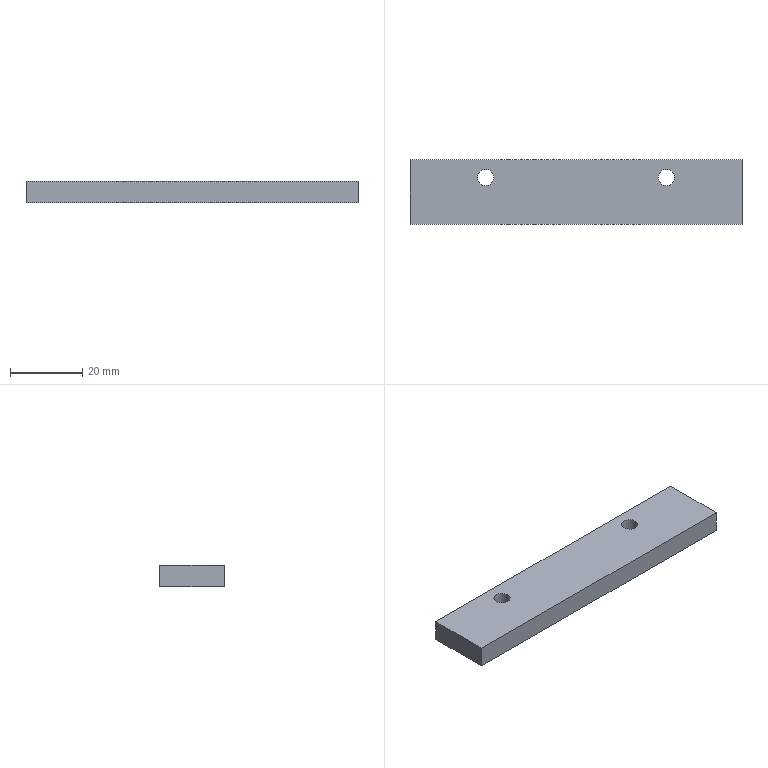Part | STEP file | 2061 Bag feed artificial stone plate A | 1 solid | 10 faces | box 92 x 18 x 6 mm | volume 9745 mm3 | plane 6 | cylinder 4 | commonest cylinder face diameters 4.5 x4
STEP:
#1=CARTESIAN_POINT('',(0.,0.,0.));
#2=DIRECTION('',(0.,0.,1.));
#3=DIRECTION('',(1.,0.,0.));
#4=AXIS2_PLACEMENT_3D('',#1,#2,#3);
#5=CARTESIAN_POINT('',(-22.75,4.,0.));
#6=VERTEX_POINT('',#5);
#7=CARTESIAN_POINT('',(-22.75,4.,6.));
#8=VERTEX_POINT('',#7);
#9=CARTESIAN_POINT('',(-22.75,4.,6.));
#10=DIRECTION('',(0.,0.,1.));
#11=VECTOR('',#10,1.);
#12=LINE('',#9,#11);
#13=CARTESIAN_POINT('',(-25.,4.,6.));
#14=DIRECTION('',(0.,0.,1.));
#15=DIRECTION('',(1.,0.,0.));
#16=AXIS2_PLACEMENT_3D('',#13,#14,#15);
#17=CYLINDRICAL_SURFACE('',#16,2.25);
#18=CARTESIAN_POINT('',(6.283,0.));
#19=DIRECTION('',(0.,1.));
#20=VECTOR('',#19,1.);
#21=LINE('',#18,#20);
#22=(GEOMETRIC_REPRESENTATION_CONTEXT(2)PARAMETRIC_REPRESENTATION_CONTEXT()REPRESENTATION_CONTEXT('',''));
#23=DEFINITIONAL_REPRESENTATION('',(#21),#22);
#24=PCURVE('',#17,#23);
#25=CARTESIAN_POINT('',(-25.,4.,6.));
#26=DIRECTION('',(0.,0.,1.));
#27=DIRECTION('',(1.,0.,0.));
#28=AXIS2_PLACEMENT_3D('',#25,#26,#27);
#29=CYLINDRICAL_SURFACE('',#28,2.25);
#30=CARTESIAN_POINT('',(0.,0.));
#31=DIRECTION('',(0.,1.));
#32=VECTOR('',#31,1.);
#33=LINE('',#30,#32);
#34=(GEOMETRIC_REPRESENTATION_CONTEXT(2)PARAMETRIC_REPRESENTATION_CONTEXT()REPRESENTATION_CONTEXT('',''));
#35=DEFINITIONAL_REPRESENTATION('',(#33),#34);
#36=PCURVE('',#29,#35);
#37=SURFACE_CURVE('',#12,(#24,#36),.PCURVE_S1.);
#38=EDGE_CURVE('',#6,#8,#37,.T.);
#39=ORIENTED_EDGE('',*,*,#38,.T.);
#40=CARTESIAN_POINT('',(-27.25,4.,6.));
#41=VERTEX_POINT('',#40);
#42=CARTESIAN_POINT('',(-25.,4.,6.));
#43=DIRECTION('',(0.,0.,1.));
#44=DIRECTION('',(1.,0.,0.));
#45=AXIS2_PLACEMENT_3D('',#42,#43,#44);
#46=CIRCLE('',#45,2.25);
#47=CARTESIAN_POINT('',(0.,0.));
#48=DIRECTION('',(1.,0.));
#49=VECTOR('',#48,1.);
#50=LINE('',#47,#49);
#51=(GEOMETRIC_REPRESENTATION_CONTEXT(2)PARAMETRIC_REPRESENTATION_CONTEXT()REPRESENTATION_CONTEXT('',''));
#52=DEFINITIONAL_REPRESENTATION('',(#50),#51);
#53=PCURVE('',#17,#52);
#54=CARTESIAN_POINT('',(0.,0.,6.));
#55=DIRECTION('',(0.,0.,-1.));
#56=DIRECTION('',(-1.,0.,0.));
#57=AXIS2_PLACEMENT_3D('',#54,#55,#56);
#58=PLANE('',#57);
#59=CARTESIAN_POINT('',(22.75,4.));
#60=CARTESIAN_POINT('',(22.75,7.897));
#61=CARTESIAN_POINT('',(26.125,5.949));
#62=CARTESIAN_POINT('',(29.5,4.));
#63=CARTESIAN_POINT('',(26.125,2.051));
#64=CARTESIAN_POINT('',(22.75,0.1029));
#65=CARTESIAN_POINT('',(22.75,4.));
#66=(BOUNDED_CURVE()B_SPLINE_CURVE(2,(#59,#60,#61,#62,#63,#64,#65),.UNSPECIFIED.,.T.,.F.)B_SPLINE_CURVE_WITH_KNOTS((1,2,2,2,2,1),(-2.094,0.,2.094,4.189,6.283,8.378),.UNSPECIFIED.)CURVE()GEOMETRIC_REPRESENTATION_ITEM()RATIONAL_B_SPLINE_CURVE((1.,0.5,1.,0.5,1.,0.5,1.))REPRESENTATION_ITEM(''));
#67=(GEOMETRIC_REPRESENTATION_CONTEXT(2)PARAMETRIC_REPRESENTATION_CONTEXT()REPRESENTATION_CONTEXT('',''));
#68=DEFINITIONAL_REPRESENTATION('',(#66),#67);
#69=PCURVE('',#58,#68);
#70=SURFACE_CURVE('',#46,(#53,#69),.PCURVE_S1.);
#71=EDGE_CURVE('',#41,#8,#70,.T.);
#72=ORIENTED_EDGE('',*,*,#71,.F.);
#73=CARTESIAN_POINT('',(-27.25,4.,0.));
#74=VERTEX_POINT('',#73);
#75=CARTESIAN_POINT('',(-27.25,4.,6.));
#76=DIRECTION('',(0.,0.,1.));
#77=VECTOR('',#76,1.);
#78=LINE('',#75,#77);
#79=CARTESIAN_POINT('',(3.142,0.));
#80=DIRECTION('',(0.,1.));
#81=VECTOR('',#80,1.);
#82=LINE('',#79,#81);
#83=(GEOMETRIC_REPRESENTATION_CONTEXT(2)PARAMETRIC_REPRESENTATION_CONTEXT()REPRESENTATION_CONTEXT('',''));
#84=DEFINITIONAL_REPRESENTATION('',(#82),#83);
#85=PCURVE('',#17,#84);
#86=CARTESIAN_POINT('',(3.142,0.));
#87=DIRECTION('',(0.,1.));
#88=VECTOR('',#87,1.);
#89=LINE('',#86,#88);
#90=(GEOMETRIC_REPRESENTATION_CONTEXT(2)PARAMETRIC_REPRESENTATION_CONTEXT()REPRESENTATION_CONTEXT('',''));
#91=DEFINITIONAL_REPRESENTATION('',(#89),#90);
#92=PCURVE('',#29,#91);
#93=SURFACE_CURVE('',#78,(#85,#92),.PCURVE_S1.);
#94=EDGE_CURVE('',#74,#41,#93,.T.);
#95=ORIENTED_EDGE('',*,*,#94,.F.);
#96=CARTESIAN_POINT('',(-25.,4.,0.));
#97=DIRECTION('',(0.,0.,-1.));
#98=DIRECTION('',(-1.,0.,0.));
#99=AXIS2_PLACEMENT_3D('',#96,#97,#98);
#100=CIRCLE('',#99,2.25);
#101=CARTESIAN_POINT('',(9.425,-6.));
#102=DIRECTION('',(-1.,0.));
#103=VECTOR('',#102,1.);
#104=LINE('',#101,#103);
#105=(GEOMETRIC_REPRESENTATION_CONTEXT(2)PARAMETRIC_REPRESENTATION_CONTEXT()REPRESENTATION_CONTEXT('',''));
#106=DEFINITIONAL_REPRESENTATION('',(#104),#105);
#107=PCURVE('',#17,#106);
#108=CARTESIAN_POINT('',(0.,0.,0.));
#109=DIRECTION('',(0.,0.,-1.));
#110=DIRECTION('',(-1.,0.,0.));
#111=AXIS2_PLACEMENT_3D('',#108,#109,#110);
#112=PLANE('',#111);
#113=CARTESIAN_POINT('',(25.,4.));
#114=DIRECTION('',(1.,0.));
#115=AXIS2_PLACEMENT_2D('',#113,#114);
#116=CIRCLE('',#115,2.25);
#117=(GEOMETRIC_REPRESENTATION_CONTEXT(2)PARAMETRIC_REPRESENTATION_CONTEXT()REPRESENTATION_CONTEXT('',''));
#118=DEFINITIONAL_REPRESENTATION('',(#116),#117);
#119=PCURVE('',#112,#118);
#120=SURFACE_CURVE('',#100,(#107,#119),.PCURVE_S1.);
#121=EDGE_CURVE('',#6,#74,#120,.T.);
#122=ORIENTED_EDGE('',*,*,#121,.F.);
#123=EDGE_LOOP('',(#39,#72,#95,#122));
#124=FACE_BOUND('',#123,.F.);
#125=ADVANCED_FACE('',(#124),#17,.F.);
#126=CARTESIAN_POINT('',(27.25,4.,0.));
#127=VERTEX_POINT('',#126);
#128=CARTESIAN_POINT('',(27.25,4.,6.));
#129=VERTEX_POINT('',#128);
#130=CARTESIAN_POINT('',(27.25,4.,6.));
#131=DIRECTION('',(0.,0.,1.));
#132=VECTOR('',#131,1.);
#133=LINE('',#130,#132);
#134=CARTESIAN_POINT('',(25.,4.,6.));
#135=DIRECTION('',(0.,0.,1.));
#136=DIRECTION('',(1.,0.,0.));
#137=AXIS2_PLACEMENT_3D('',#134,#135,#136);
#138=CYLINDRICAL_SURFACE('',#137,2.25);
#139=CARTESIAN_POINT('',(6.283,0.));
#140=DIRECTION('',(0.,1.));
#141=VECTOR('',#140,1.);
#142=LINE('',#139,#141);
#143=(GEOMETRIC_REPRESENTATION_CONTEXT(2)PARAMETRIC_REPRESENTATION_CONTEXT()REPRESENTATION_CONTEXT('',''));
#144=DEFINITIONAL_REPRESENTATION('',(#142),#143);
#145=PCURVE('',#138,#144);
#146=CARTESIAN_POINT('',(25.,4.,6.));
#147=DIRECTION('',(0.,0.,1.));
#148=DIRECTION('',(1.,0.,0.));
#149=AXIS2_PLACEMENT_3D('',#146,#147,#148);
#150=CYLINDRICAL_SURFACE('',#149,2.25);
#151=CARTESIAN_POINT('',(0.,0.));
#152=DIRECTION('',(0.,1.));
#153=VECTOR('',#152,1.);
#154=LINE('',#151,#153);
#155=(GEOMETRIC_REPRESENTATION_CONTEXT(2)PARAMETRIC_REPRESENTATION_CONTEXT()REPRESENTATION_CONTEXT('',''));
#156=DEFINITIONAL_REPRESENTATION('',(#154),#155);
#157=PCURVE('',#150,#156);
#158=SURFACE_CURVE('',#133,(#145,#157),.PCURVE_S1.);
#159=EDGE_CURVE('',#127,#129,#158,.T.);
#160=ORIENTED_EDGE('',*,*,#159,.T.);
#161=CARTESIAN_POINT('',(22.75,4.,6.));
#162=VERTEX_POINT('',#161);
#163=CARTESIAN_POINT('',(25.,4.,6.));
#164=DIRECTION('',(0.,0.,1.));
#165=DIRECTION('',(1.,0.,0.));
#166=AXIS2_PLACEMENT_3D('',#163,#164,#165);
#167=CIRCLE('',#166,2.25);
#168=CARTESIAN_POINT('',(0.,0.));
#169=DIRECTION('',(1.,0.));
#170=VECTOR('',#169,1.);
#171=LINE('',#168,#170);
#172=(GEOMETRIC_REPRESENTATION_CONTEXT(2)PARAMETRIC_REPRESENTATION_CONTEXT()REPRESENTATION_CONTEXT('',''));
#173=DEFINITIONAL_REPRESENTATION('',(#171),#172);
#174=PCURVE('',#138,#173);
#175=CARTESIAN_POINT('',(-27.25,4.));
#176=CARTESIAN_POINT('',(-27.25,7.897));
#177=CARTESIAN_POINT('',(-23.875,5.949));
#178=CARTESIAN_POINT('',(-20.5,4.));
#179=CARTESIAN_POINT('',(-23.875,2.051));
#180=CARTESIAN_POINT('',(-27.25,0.1029));
#181=CARTESIAN_POINT('',(-27.25,4.));
#182=(BOUNDED_CURVE()B_SPLINE_CURVE(2,(#175,#176,#177,#178,#179,#180,#181),.UNSPECIFIED.,.T.,.F.)B_SPLINE_CURVE_WITH_KNOTS((1,2,2,2,2,1),(-2.094,0.,2.094,4.189,6.283,8.378),.UNSPECIFIED.)CURVE()GEOMETRIC_REPRESENTATION_ITEM()RATIONAL_B_SPLINE_CURVE((1.,0.5,1.,0.5,1.,0.5,1.))REPRESENTATION_ITEM(''));
#183=(GEOMETRIC_REPRESENTATION_CONTEXT(2)PARAMETRIC_REPRESENTATION_CONTEXT()REPRESENTATION_CONTEXT('',''));
#184=DEFINITIONAL_REPRESENTATION('',(#182),#183);
#185=PCURVE('',#58,#184);
#186=SURFACE_CURVE('',#167,(#174,#185),.PCURVE_S1.);
#187=EDGE_CURVE('',#162,#129,#186,.T.);
#188=ORIENTED_EDGE('',*,*,#187,.F.);
#189=CARTESIAN_POINT('',(22.75,4.,0.));
#190=VERTEX_POINT('',#189);
#191=CARTESIAN_POINT('',(22.75,4.,6.));
#192=DIRECTION('',(0.,0.,1.));
#193=VECTOR('',#192,1.);
#194=LINE('',#191,#193);
#195=CARTESIAN_POINT('',(3.142,0.));
#196=DIRECTION('',(0.,1.));
#197=VECTOR('',#196,1.);
#198=LINE('',#195,#197);
#199=(GEOMETRIC_REPRESENTATION_CONTEXT(2)PARAMETRIC_REPRESENTATION_CONTEXT()REPRESENTATION_CONTEXT('',''));
#200=DEFINITIONAL_REPRESENTATION('',(#198),#199);
#201=PCURVE('',#138,#200);
#202=CARTESIAN_POINT('',(3.142,0.));
#203=DIRECTION('',(0.,1.));
#204=VECTOR('',#203,1.);
#205=LINE('',#202,#204);
#206=(GEOMETRIC_REPRESENTATION_CONTEXT(2)PARAMETRIC_REPRESENTATION_CONTEXT()REPRESENTATION_CONTEXT('',''));
#207=DEFINITIONAL_REPRESENTATION('',(#205),#206);
#208=PCURVE('',#150,#207);
#209=SURFACE_CURVE('',#194,(#201,#208),.PCURVE_S1.);
#210=EDGE_CURVE('',#190,#162,#209,.T.);
#211=ORIENTED_EDGE('',*,*,#210,.F.);
#212=CARTESIAN_POINT('',(25.,4.,0.));
#213=DIRECTION('',(0.,0.,-1.));
#214=DIRECTION('',(-1.,0.,0.));
#215=AXIS2_PLACEMENT_3D('',#212,#213,#214);
#216=CIRCLE('',#215,2.25);
#217=CARTESIAN_POINT('',(9.425,-6.));
#218=DIRECTION('',(-1.,0.));
#219=VECTOR('',#218,1.);
#220=LINE('',#217,#219);
#221=(GEOMETRIC_REPRESENTATION_CONTEXT(2)PARAMETRIC_REPRESENTATION_CONTEXT()REPRESENTATION_CONTEXT('',''));
#222=DEFINITIONAL_REPRESENTATION('',(#220),#221);
#223=PCURVE('',#138,#222);
#224=CARTESIAN_POINT('',(-25.,4.));
#225=DIRECTION('',(1.,0.));
#226=AXIS2_PLACEMENT_2D('',#224,#225);
#227=CIRCLE('',#226,2.25);
#228=(GEOMETRIC_REPRESENTATION_CONTEXT(2)PARAMETRIC_REPRESENTATION_CONTEXT()REPRESENTATION_CONTEXT('',''));
#229=DEFINITIONAL_REPRESENTATION('',(#227),#228);
#230=PCURVE('',#112,#229);
#231=SURFACE_CURVE('',#216,(#223,#230),.PCURVE_S1.);
#232=EDGE_CURVE('',#127,#190,#231,.T.);
#233=ORIENTED_EDGE('',*,*,#232,.F.);
#234=EDGE_LOOP('',(#160,#188,#211,#233));
#235=FACE_BOUND('',#234,.F.);
#236=ADVANCED_FACE('',(#235),#138,.F.);
#237=CARTESIAN_POINT('',(46.,-9.,0.));
#238=VERTEX_POINT('',#237);
#239=CARTESIAN_POINT('',(46.,9.,0.));
#240=VERTEX_POINT('',#239);
#241=CARTESIAN_POINT('',(46.,-9.,0.));
#242=DIRECTION('',(0.,1.,0.));
#243=VECTOR('',#242,1.);
#244=LINE('',#241,#243);
#245=CARTESIAN_POINT('',(46.,-9.,6.));
#246=DIRECTION('',(-1.,0.,0.));
#247=DIRECTION('',(0.,0.,1.));
#248=AXIS2_PLACEMENT_3D('',#245,#246,#247);
#249=PLANE('',#248);
#250=CARTESIAN_POINT('',(-6.,0.));
#251=DIRECTION('',(0.,1.));
#252=VECTOR('',#251,1.);
#253=LINE('',#250,#252);
#254=(GEOMETRIC_REPRESENTATION_CONTEXT(2)PARAMETRIC_REPRESENTATION_CONTEXT()REPRESENTATION_CONTEXT('',''));
#255=DEFINITIONAL_REPRESENTATION('',(#253),#254);
#256=PCURVE('',#249,#255);
#257=CARTESIAN_POINT('',(-46.,-9.));
#258=DIRECTION('',(0.,1.));
#259=VECTOR('',#258,1.);
#260=LINE('',#257,#259);
#261=(GEOMETRIC_REPRESENTATION_CONTEXT(2)PARAMETRIC_REPRESENTATION_CONTEXT()REPRESENTATION_CONTEXT('',''));
#262=DEFINITIONAL_REPRESENTATION('',(#260),#261);
#263=PCURVE('',#112,#262);
#264=SURFACE_CURVE('',#244,(#256,#263),.PCURVE_S1.);
#265=EDGE_CURVE('',#238,#240,#264,.T.);
#266=ORIENTED_EDGE('',*,*,#265,.T.);
#267=CARTESIAN_POINT('',(46.,9.,6.));
#268=VERTEX_POINT('',#267);
#269=CARTESIAN_POINT('',(46.,9.,6.));
#270=DIRECTION('',(0.,0.,-1.));
#271=VECTOR('',#270,1.);
#272=LINE('',#269,#271);
#273=CARTESIAN_POINT('',(0.,18.));
#274=DIRECTION('',(-1.,0.));
#275=VECTOR('',#274,1.);
#276=LINE('',#273,#275);
#277=(GEOMETRIC_REPRESENTATION_CONTEXT(2)PARAMETRIC_REPRESENTATION_CONTEXT()REPRESENTATION_CONTEXT('',''));
#278=DEFINITIONAL_REPRESENTATION('',(#276),#277);
#279=PCURVE('',#249,#278);
#280=CARTESIAN_POINT('',(-46.,9.,6.));
#281=DIRECTION('',(0.,-1.,0.));
#282=DIRECTION('',(0.,0.,-1.));
#283=AXIS2_PLACEMENT_3D('',#280,#281,#282);
#284=PLANE('',#283);
#285=CARTESIAN_POINT('',(0.,92.));
#286=DIRECTION('',(1.,0.));
#287=VECTOR('',#286,1.);
#288=LINE('',#285,#287);
#289=(GEOMETRIC_REPRESENTATION_CONTEXT(2)PARAMETRIC_REPRESENTATION_CONTEXT()REPRESENTATION_CONTEXT('',''));
#290=DEFINITIONAL_REPRESENTATION('',(#288),#289);
#291=PCURVE('',#284,#290);
#292=SURFACE_CURVE('',#272,(#279,#291),.PCURVE_S1.);
#293=EDGE_CURVE('',#268,#240,#292,.T.);
#294=ORIENTED_EDGE('',*,*,#293,.F.);
#295=CARTESIAN_POINT('',(46.,-9.,6.));
#296=VERTEX_POINT('',#295);
#297=CARTESIAN_POINT('',(46.,-9.,6.));
#298=DIRECTION('',(0.,1.,0.));
#299=VECTOR('',#298,1.);
#300=LINE('',#297,#299);
#301=CARTESIAN_POINT('',(0.,0.));
#302=DIRECTION('',(0.,1.));
#303=VECTOR('',#302,1.);
#304=LINE('',#301,#303);
#305=(GEOMETRIC_REPRESENTATION_CONTEXT(2)PARAMETRIC_REPRESENTATION_CONTEXT()REPRESENTATION_CONTEXT('',''));
#306=DEFINITIONAL_REPRESENTATION('',(#304),#305);
#307=PCURVE('',#249,#306);
#308=CARTESIAN_POINT('',(-46.,-9.));
#309=DIRECTION('',(0.,1.));
#310=VECTOR('',#309,1.);
#311=LINE('',#308,#310);
#312=(GEOMETRIC_REPRESENTATION_CONTEXT(2)PARAMETRIC_REPRESENTATION_CONTEXT()REPRESENTATION_CONTEXT('',''));
#313=DEFINITIONAL_REPRESENTATION('',(#311),#312);
#314=PCURVE('',#58,#313);
#315=SURFACE_CURVE('',#300,(#307,#314),.PCURVE_S1.);
#316=EDGE_CURVE('',#296,#268,#315,.T.);
#317=ORIENTED_EDGE('',*,*,#316,.F.);
#318=CARTESIAN_POINT('',(46.,-9.,6.));
#319=DIRECTION('',(0.,0.,-1.));
#320=VECTOR('',#319,1.);
#321=LINE('',#318,#320);
#322=CARTESIAN_POINT('',(0.,0.));
#323=DIRECTION('',(-1.,0.));
#324=VECTOR('',#323,1.);
#325=LINE('',#322,#324);
#326=(GEOMETRIC_REPRESENTATION_CONTEXT(2)PARAMETRIC_REPRESENTATION_CONTEXT()REPRESENTATION_CONTEXT('',''));
#327=DEFINITIONAL_REPRESENTATION('',(#325),#326);
#328=PCURVE('',#249,#327);
#329=CARTESIAN_POINT('',(-46.,-9.,6.));
#330=DIRECTION('',(0.,1.,0.));
#331=DIRECTION('',(0.,0.,1.));
#332=AXIS2_PLACEMENT_3D('',#329,#330,#331);
#333=PLANE('',#332);
#334=CARTESIAN_POINT('',(0.,92.));
#335=DIRECTION('',(-1.,0.));
#336=VECTOR('',#335,1.);
#337=LINE('',#334,#336);
#338=(GEOMETRIC_REPRESENTATION_CONTEXT(2)PARAMETRIC_REPRESENTATION_CONTEXT()REPRESENTATION_CONTEXT('',''));
#339=DEFINITIONAL_REPRESENTATION('',(#337),#338);
#340=PCURVE('',#333,#339);
#341=SURFACE_CURVE('',#321,(#328,#340),.PCURVE_S1.);
#342=EDGE_CURVE('',#296,#238,#341,.T.);
#343=ORIENTED_EDGE('',*,*,#342,.T.);
#344=EDGE_LOOP('',(#266,#294,#317,#343));
#345=FACE_BOUND('',#344,.T.);
#346=ADVANCED_FACE('',(#345),#249,.F.);
#347=CARTESIAN_POINT('',(-46.,9.,0.));
#348=VERTEX_POINT('',#347);
#349=CARTESIAN_POINT('',(-46.,9.,0.));
#350=DIRECTION('',(-1.,0.,0.));
#351=VECTOR('',#350,1.);
#352=LINE('',#349,#351);
#353=CARTESIAN_POINT('',(6.,0.));
#354=DIRECTION('',(0.,-1.));
#355=VECTOR('',#354,1.);
#356=LINE('',#353,#355);
#357=(GEOMETRIC_REPRESENTATION_CONTEXT(2)PARAMETRIC_REPRESENTATION_CONTEXT()REPRESENTATION_CONTEXT('',''));
#358=DEFINITIONAL_REPRESENTATION('',(#356),#357);
#359=PCURVE('',#284,#358);
#360=CARTESIAN_POINT('',(46.,9.));
#361=DIRECTION('',(1.,0.));
#362=VECTOR('',#361,1.);
#363=LINE('',#360,#362);
#364=(GEOMETRIC_REPRESENTATION_CONTEXT(2)PARAMETRIC_REPRESENTATION_CONTEXT()REPRESENTATION_CONTEXT('',''));
#365=DEFINITIONAL_REPRESENTATION('',(#363),#364);
#366=PCURVE('',#112,#365);
#367=SURFACE_CURVE('',#352,(#359,#366),.PCURVE_S1.);
#368=EDGE_CURVE('',#240,#348,#367,.T.);
#369=ORIENTED_EDGE('',*,*,#368,.T.);
#370=CARTESIAN_POINT('',(-46.,9.,6.));
#371=VERTEX_POINT('',#370);
#372=CARTESIAN_POINT('',(-46.,9.,6.));
#373=DIRECTION('',(0.,0.,-1.));
#374=VECTOR('',#373,1.);
#375=LINE('',#372,#374);
#376=CARTESIAN_POINT('',(0.,0.));
#377=DIRECTION('',(1.,0.));
#378=VECTOR('',#377,1.);
#379=LINE('',#376,#378);
#380=(GEOMETRIC_REPRESENTATION_CONTEXT(2)PARAMETRIC_REPRESENTATION_CONTEXT()REPRESENTATION_CONTEXT('',''));
#381=DEFINITIONAL_REPRESENTATION('',(#379),#380);
#382=PCURVE('',#284,#381);
#383=CARTESIAN_POINT('',(-46.,-9.,6.));
#384=DIRECTION('',(1.,0.,0.));
#385=DIRECTION('',(0.,0.,-1.));
#386=AXIS2_PLACEMENT_3D('',#383,#384,#385);
#387=PLANE('',#386);
#388=CARTESIAN_POINT('',(0.,18.));
#389=DIRECTION('',(1.,0.));
#390=VECTOR('',#389,1.);
#391=LINE('',#388,#390);
#392=(GEOMETRIC_REPRESENTATION_CONTEXT(2)PARAMETRIC_REPRESENTATION_CONTEXT()REPRESENTATION_CONTEXT('',''));
#393=DEFINITIONAL_REPRESENTATION('',(#391),#392);
#394=PCURVE('',#387,#393);
#395=SURFACE_CURVE('',#375,(#382,#394),.PCURVE_S1.);
#396=EDGE_CURVE('',#371,#348,#395,.T.);
#397=ORIENTED_EDGE('',*,*,#396,.F.);
#398=CARTESIAN_POINT('',(-46.,9.,6.));
#399=DIRECTION('',(-1.,0.,0.));
#400=VECTOR('',#399,1.);
#401=LINE('',#398,#400);
#402=CARTESIAN_POINT('',(0.,0.));
#403=DIRECTION('',(0.,-1.));
#404=VECTOR('',#403,1.);
#405=LINE('',#402,#404);
#406=(GEOMETRIC_REPRESENTATION_CONTEXT(2)PARAMETRIC_REPRESENTATION_CONTEXT()REPRESENTATION_CONTEXT('',''));
#407=DEFINITIONAL_REPRESENTATION('',(#405),#406);
#408=PCURVE('',#284,#407);
#409=CARTESIAN_POINT('',(46.,9.));
#410=DIRECTION('',(1.,0.));
#411=VECTOR('',#410,1.);
#412=LINE('',#409,#411);
#413=(GEOMETRIC_REPRESENTATION_CONTEXT(2)PARAMETRIC_REPRESENTATION_CONTEXT()REPRESENTATION_CONTEXT('',''));
#414=DEFINITIONAL_REPRESENTATION('',(#412),#413);
#415=PCURVE('',#58,#414);
#416=SURFACE_CURVE('',#401,(#408,#415),.PCURVE_S1.);
#417=EDGE_CURVE('',#268,#371,#416,.T.);
#418=ORIENTED_EDGE('',*,*,#417,.F.);
#419=ORIENTED_EDGE('',*,*,#293,.T.);
#420=EDGE_LOOP('',(#369,#397,#418,#419));
#421=FACE_BOUND('',#420,.T.);
#422=ADVANCED_FACE('',(#421),#284,.F.);
#423=CARTESIAN_POINT('',(-46.,-9.,0.));
#424=VERTEX_POINT('',#423);
#425=CARTESIAN_POINT('',(-46.,-9.,0.));
#426=DIRECTION('',(0.,-1.,0.));
#427=VECTOR('',#426,1.);
#428=LINE('',#425,#427);
#429=CARTESIAN_POINT('',(6.,0.));
#430=DIRECTION('',(0.,-1.));
#431=VECTOR('',#430,1.);
#432=LINE('',#429,#431);
#433=(GEOMETRIC_REPRESENTATION_CONTEXT(2)PARAMETRIC_REPRESENTATION_CONTEXT()REPRESENTATION_CONTEXT('',''));
#434=DEFINITIONAL_REPRESENTATION('',(#432),#433);
#435=PCURVE('',#387,#434);
#436=CARTESIAN_POINT('',(46.,-9.));
#437=DIRECTION('',(0.,-1.));
#438=VECTOR('',#437,1.);
#439=LINE('',#436,#438);
#440=(GEOMETRIC_REPRESENTATION_CONTEXT(2)PARAMETRIC_REPRESENTATION_CONTEXT()REPRESENTATION_CONTEXT('',''));
#441=DEFINITIONAL_REPRESENTATION('',(#439),#440);
#442=PCURVE('',#112,#441);
#443=SURFACE_CURVE('',#428,(#435,#442),.PCURVE_S1.);
#444=EDGE_CURVE('',#348,#424,#443,.T.);
#445=ORIENTED_EDGE('',*,*,#444,.T.);
#446=CARTESIAN_POINT('',(-46.,-9.,6.));
#447=VERTEX_POINT('',#446);
#448=CARTESIAN_POINT('',(-46.,-9.,6.));
#449=DIRECTION('',(0.,0.,-1.));
#450=VECTOR('',#449,1.);
#451=LINE('',#448,#450);
#452=CARTESIAN_POINT('',(0.,0.));
#453=DIRECTION('',(1.,0.));
#454=VECTOR('',#453,1.);
#455=LINE('',#452,#454);
#456=(GEOMETRIC_REPRESENTATION_CONTEXT(2)PARAMETRIC_REPRESENTATION_CONTEXT()REPRESENTATION_CONTEXT('',''));
#457=DEFINITIONAL_REPRESENTATION('',(#455),#456);
#458=PCURVE('',#387,#457);
#459=CARTESIAN_POINT('',(0.,0.));
#460=DIRECTION('',(-1.,0.));
#461=VECTOR('',#460,1.);
#462=LINE('',#459,#461);
#463=(GEOMETRIC_REPRESENTATION_CONTEXT(2)PARAMETRIC_REPRESENTATION_CONTEXT()REPRESENTATION_CONTEXT('',''));
#464=DEFINITIONAL_REPRESENTATION('',(#462),#463);
#465=PCURVE('',#333,#464);
#466=SURFACE_CURVE('',#451,(#458,#465),.PCURVE_S1.);
#467=EDGE_CURVE('',#447,#424,#466,.T.);
#468=ORIENTED_EDGE('',*,*,#467,.F.);
#469=CARTESIAN_POINT('',(-46.,-9.,6.));
#470=DIRECTION('',(0.,-1.,0.));
#471=VECTOR('',#470,1.);
#472=LINE('',#469,#471);
#473=CARTESIAN_POINT('',(0.,0.));
#474=DIRECTION('',(0.,-1.));
#475=VECTOR('',#474,1.);
#476=LINE('',#473,#475);
#477=(GEOMETRIC_REPRESENTATION_CONTEXT(2)PARAMETRIC_REPRESENTATION_CONTEXT()REPRESENTATION_CONTEXT('',''));
#478=DEFINITIONAL_REPRESENTATION('',(#476),#477);
#479=PCURVE('',#387,#478);
#480=CARTESIAN_POINT('',(46.,-9.));
#481=DIRECTION('',(0.,-1.));
#482=VECTOR('',#481,1.);
#483=LINE('',#480,#482);
#484=(GEOMETRIC_REPRESENTATION_CONTEXT(2)PARAMETRIC_REPRESENTATION_CONTEXT()REPRESENTATION_CONTEXT('',''));
#485=DEFINITIONAL_REPRESENTATION('',(#483),#484);
#486=PCURVE('',#58,#485);
#487=SURFACE_CURVE('',#472,(#479,#486),.PCURVE_S1.);
#488=EDGE_CURVE('',#371,#447,#487,.T.);
#489=ORIENTED_EDGE('',*,*,#488,.F.);
#490=ORIENTED_EDGE('',*,*,#396,.T.);
#491=EDGE_LOOP('',(#445,#468,#489,#490));
#492=FACE_BOUND('',#491,.T.);
#493=ADVANCED_FACE('',(#492),#387,.F.);
#494=CARTESIAN_POINT('',(-46.,-9.,0.));
#495=DIRECTION('',(1.,0.,0.));
#496=VECTOR('',#495,1.);
#497=LINE('',#494,#496);
#498=CARTESIAN_POINT('',(-6.,0.));
#499=DIRECTION('',(0.,1.));
#500=VECTOR('',#499,1.);
#501=LINE('',#498,#500);
#502=(GEOMETRIC_REPRESENTATION_CONTEXT(2)PARAMETRIC_REPRESENTATION_CONTEXT()REPRESENTATION_CONTEXT('',''));
#503=DEFINITIONAL_REPRESENTATION('',(#501),#502);
#504=PCURVE('',#333,#503);
#505=CARTESIAN_POINT('',(46.,-9.));
#506=DIRECTION('',(-1.,0.));
#507=VECTOR('',#506,1.);
#508=LINE('',#505,#507);
#509=(GEOMETRIC_REPRESENTATION_CONTEXT(2)PARAMETRIC_REPRESENTATION_CONTEXT()REPRESENTATION_CONTEXT('',''));
#510=DEFINITIONAL_REPRESENTATION('',(#508),#509);
#511=PCURVE('',#112,#510);
#512=SURFACE_CURVE('',#497,(#504,#511),.PCURVE_S1.);
#513=EDGE_CURVE('',#424,#238,#512,.T.);
#514=ORIENTED_EDGE('',*,*,#513,.T.);
#515=ORIENTED_EDGE('',*,*,#342,.F.);
#516=CARTESIAN_POINT('',(-46.,-9.,6.));
#517=DIRECTION('',(1.,0.,0.));
#518=VECTOR('',#517,1.);
#519=LINE('',#516,#518);
#520=CARTESIAN_POINT('',(0.,0.));
#521=DIRECTION('',(0.,1.));
#522=VECTOR('',#521,1.);
#523=LINE('',#520,#522);
#524=(GEOMETRIC_REPRESENTATION_CONTEXT(2)PARAMETRIC_REPRESENTATION_CONTEXT()REPRESENTATION_CONTEXT('',''));
#525=DEFINITIONAL_REPRESENTATION('',(#523),#524);
#526=PCURVE('',#333,#525);
#527=CARTESIAN_POINT('',(46.,-9.));
#528=DIRECTION('',(-1.,0.));
#529=VECTOR('',#528,1.);
#530=LINE('',#527,#529);
#531=(GEOMETRIC_REPRESENTATION_CONTEXT(2)PARAMETRIC_REPRESENTATION_CONTEXT()REPRESENTATION_CONTEXT('',''));
#532=DEFINITIONAL_REPRESENTATION('',(#530),#531);
#533=PCURVE('',#58,#532);
#534=SURFACE_CURVE('',#519,(#526,#533),.PCURVE_S1.);
#535=EDGE_CURVE('',#447,#296,#534,.T.);
#536=ORIENTED_EDGE('',*,*,#535,.F.);
#537=ORIENTED_EDGE('',*,*,#467,.T.);
#538=EDGE_LOOP('',(#514,#515,#536,#537));
#539=FACE_BOUND('',#538,.T.);
#540=ADVANCED_FACE('',(#539),#333,.F.);
#541=CARTESIAN_POINT('',(-25.,4.,6.));
#542=DIRECTION('',(0.,0.,1.));
#543=DIRECTION('',(1.,0.,0.));
#544=AXIS2_PLACEMENT_3D('',#541,#542,#543);
#545=CIRCLE('',#544,2.25);
#546=CARTESIAN_POINT('',(22.75,4.));
#547=CARTESIAN_POINT('',(22.75,7.897));
#548=CARTESIAN_POINT('',(26.125,5.949));
#549=CARTESIAN_POINT('',(29.5,4.));
#550=CARTESIAN_POINT('',(26.125,2.051));
#551=CARTESIAN_POINT('',(22.75,0.1029));
#552=CARTESIAN_POINT('',(22.75,4.));
#553=(BOUNDED_CURVE()B_SPLINE_CURVE(2,(#546,#547,#548,#549,#550,#551,#552),.UNSPECIFIED.,.T.,.F.)B_SPLINE_CURVE_WITH_KNOTS((1,2,2,2,2,1),(-2.094,0.,2.094,4.189,6.283,8.378),.UNSPECIFIED.)CURVE()GEOMETRIC_REPRESENTATION_ITEM()RATIONAL_B_SPLINE_CURVE((1.,0.5,1.,0.5,1.,0.5,1.))REPRESENTATION_ITEM(''));
#554=(GEOMETRIC_REPRESENTATION_CONTEXT(2)PARAMETRIC_REPRESENTATION_CONTEXT()REPRESENTATION_CONTEXT('',''));
#555=DEFINITIONAL_REPRESENTATION('',(#553),#554);
#556=PCURVE('',#58,#555);
#557=CARTESIAN_POINT('',(0.,0.));
#558=DIRECTION('',(1.,0.));
#559=VECTOR('',#558,1.);
#560=LINE('',#557,#559);
#561=(GEOMETRIC_REPRESENTATION_CONTEXT(2)PARAMETRIC_REPRESENTATION_CONTEXT()REPRESENTATION_CONTEXT('',''));
#562=DEFINITIONAL_REPRESENTATION('',(#560),#561);
#563=PCURVE('',#29,#562);
#564=SURFACE_CURVE('',#545,(#556,#563),.PCURVE_S1.);
#565=EDGE_CURVE('',#8,#41,#564,.T.);
#566=ORIENTED_EDGE('',*,*,#565,.F.);
#567=ORIENTED_EDGE('',*,*,#71,.F.);
#568=EDGE_LOOP('',(#566,#567));
#569=FACE_BOUND('',#568,.T.);
#570=CARTESIAN_POINT('',(25.,4.,6.));
#571=DIRECTION('',(0.,0.,1.));
#572=DIRECTION('',(1.,0.,0.));
#573=AXIS2_PLACEMENT_3D('',#570,#571,#572);
#574=CIRCLE('',#573,2.25);
#575=CARTESIAN_POINT('',(-27.25,4.));
#576=CARTESIAN_POINT('',(-27.25,7.897));
#577=CARTESIAN_POINT('',(-23.875,5.949));
#578=CARTESIAN_POINT('',(-20.5,4.));
#579=CARTESIAN_POINT('',(-23.875,2.051));
#580=CARTESIAN_POINT('',(-27.25,0.1029));
#581=CARTESIAN_POINT('',(-27.25,4.));
#582=(BOUNDED_CURVE()B_SPLINE_CURVE(2,(#575,#576,#577,#578,#579,#580,#581),.UNSPECIFIED.,.T.,.F.)B_SPLINE_CURVE_WITH_KNOTS((1,2,2,2,2,1),(-2.094,0.,2.094,4.189,6.283,8.378),.UNSPECIFIED.)CURVE()GEOMETRIC_REPRESENTATION_ITEM()RATIONAL_B_SPLINE_CURVE((1.,0.5,1.,0.5,1.,0.5,1.))REPRESENTATION_ITEM(''));
#583=(GEOMETRIC_REPRESENTATION_CONTEXT(2)PARAMETRIC_REPRESENTATION_CONTEXT()REPRESENTATION_CONTEXT('',''));
#584=DEFINITIONAL_REPRESENTATION('',(#582),#583);
#585=PCURVE('',#58,#584);
#586=CARTESIAN_POINT('',(0.,0.));
#587=DIRECTION('',(1.,0.));
#588=VECTOR('',#587,1.);
#589=LINE('',#586,#588);
#590=(GEOMETRIC_REPRESENTATION_CONTEXT(2)PARAMETRIC_REPRESENTATION_CONTEXT()REPRESENTATION_CONTEXT('',''));
#591=DEFINITIONAL_REPRESENTATION('',(#589),#590);
#592=PCURVE('',#150,#591);
#593=SURFACE_CURVE('',#574,(#585,#592),.PCURVE_S1.);
#594=EDGE_CURVE('',#129,#162,#593,.T.);
#595=ORIENTED_EDGE('',*,*,#594,.F.);
#596=ORIENTED_EDGE('',*,*,#187,.F.);
#597=EDGE_LOOP('',(#595,#596));
#598=FACE_BOUND('',#597,.T.);
#599=ORIENTED_EDGE('',*,*,#316,.T.);
#600=ORIENTED_EDGE('',*,*,#417,.T.);
#601=ORIENTED_EDGE('',*,*,#488,.T.);
#602=ORIENTED_EDGE('',*,*,#535,.T.);
#603=EDGE_LOOP('',(#599,#600,#601,#602));
#604=FACE_BOUND('',#603,.T.);
#605=ADVANCED_FACE('',(#569,#598,#604),#58,.F.);
#606=ORIENTED_EDGE('',*,*,#121,.F.);
#607=CARTESIAN_POINT('',(-25.,4.,0.));
#608=DIRECTION('',(0.,0.,-1.));
#609=DIRECTION('',(-1.,0.,0.));
#610=AXIS2_PLACEMENT_3D('',#607,#608,#609);
#611=CIRCLE('',#610,2.25);
#612=CARTESIAN_POINT('',(25.,4.));
#613=DIRECTION('',(1.,0.));
#614=AXIS2_PLACEMENT_2D('',#612,#613);
#615=CIRCLE('',#614,2.25);
#616=(GEOMETRIC_REPRESENTATION_CONTEXT(2)PARAMETRIC_REPRESENTATION_CONTEXT()REPRESENTATION_CONTEXT('',''));
#617=DEFINITIONAL_REPRESENTATION('',(#615),#616);
#618=PCURVE('',#112,#617);
#619=CARTESIAN_POINT('',(3.142,-6.));
#620=DIRECTION('',(-1.,0.));
#621=VECTOR('',#620,1.);
#622=LINE('',#619,#621);
#623=(GEOMETRIC_REPRESENTATION_CONTEXT(2)PARAMETRIC_REPRESENTATION_CONTEXT()REPRESENTATION_CONTEXT('',''));
#624=DEFINITIONAL_REPRESENTATION('',(#622),#623);
#625=PCURVE('',#29,#624);
#626=SURFACE_CURVE('',#611,(#618,#625),.PCURVE_S1.);
#627=EDGE_CURVE('',#74,#6,#626,.T.);
#628=ORIENTED_EDGE('',*,*,#627,.F.);
#629=EDGE_LOOP('',(#606,#628));
#630=FACE_BOUND('',#629,.T.);
#631=ORIENTED_EDGE('',*,*,#232,.F.);
#632=CARTESIAN_POINT('',(25.,4.,0.));
#633=DIRECTION('',(0.,0.,-1.));
#634=DIRECTION('',(-1.,0.,0.));
#635=AXIS2_PLACEMENT_3D('',#632,#633,#634);
#636=CIRCLE('',#635,2.25);
#637=CARTESIAN_POINT('',(-25.,4.));
#638=DIRECTION('',(1.,0.));
#639=AXIS2_PLACEMENT_2D('',#637,#638);
#640=CIRCLE('',#639,2.25);
#641=(GEOMETRIC_REPRESENTATION_CONTEXT(2)PARAMETRIC_REPRESENTATION_CONTEXT()REPRESENTATION_CONTEXT('',''));
#642=DEFINITIONAL_REPRESENTATION('',(#640),#641);
#643=PCURVE('',#112,#642);
#644=CARTESIAN_POINT('',(3.142,-6.));
#645=DIRECTION('',(-1.,0.));
#646=VECTOR('',#645,1.);
#647=LINE('',#644,#646);
#648=(GEOMETRIC_REPRESENTATION_CONTEXT(2)PARAMETRIC_REPRESENTATION_CONTEXT()REPRESENTATION_CONTEXT('',''));
#649=DEFINITIONAL_REPRESENTATION('',(#647),#648);
#650=PCURVE('',#150,#649);
#651=SURFACE_CURVE('',#636,(#643,#650),.PCURVE_S1.);
#652=EDGE_CURVE('',#190,#127,#651,.T.);
#653=ORIENTED_EDGE('',*,*,#652,.F.);
#654=EDGE_LOOP('',(#631,#653));
#655=FACE_BOUND('',#654,.T.);
#656=ORIENTED_EDGE('',*,*,#265,.F.);
#657=ORIENTED_EDGE('',*,*,#513,.F.);
#658=ORIENTED_EDGE('',*,*,#444,.F.);
#659=ORIENTED_EDGE('',*,*,#368,.F.);
#660=EDGE_LOOP('',(#656,#657,#658,#659));
#661=FACE_BOUND('',#660,.T.);
#662=ADVANCED_FACE('',(#630,#655,#661),#112,.T.);
#663=ORIENTED_EDGE('',*,*,#594,.F.);
#664=ORIENTED_EDGE('',*,*,#159,.F.);
#665=ORIENTED_EDGE('',*,*,#652,.F.);
#666=ORIENTED_EDGE('',*,*,#210,.T.);
#667=EDGE_LOOP('',(#663,#664,#665,#666));
#668=FACE_BOUND('',#667,.F.);
#669=ADVANCED_FACE('',(#668),#150,.F.);
#670=ORIENTED_EDGE('',*,*,#565,.F.);
#671=ORIENTED_EDGE('',*,*,#38,.F.);
#672=ORIENTED_EDGE('',*,*,#627,.F.);
#673=ORIENTED_EDGE('',*,*,#94,.T.);
#674=EDGE_LOOP('',(#670,#671,#672,#673));
#675=FACE_BOUND('',#674,.F.);
#676=ADVANCED_FACE('',(#675),#29,.F.);
#677=CLOSED_SHELL('',(#125,#236,#346,#422,#493,#540,#605,#662,#669,#676));
#678=MANIFOLD_SOLID_BREP('',#677);
#679=(LENGTH_UNIT()NAMED_UNIT(*)SI_UNIT(.MILLI.,.METRE.));
#680=UNCERTAINTY_MEASURE_WITH_UNIT(LENGTH_MEASURE(0.0000001),#679,'','');
#681=(NAMED_UNIT(*)PLANE_ANGLE_UNIT()SI_UNIT($,.RADIAN.));
#682=(NAMED_UNIT(*)SI_UNIT($,.STERADIAN.)SOLID_ANGLE_UNIT());
#683=(GEOMETRIC_REPRESENTATION_CONTEXT(3)GLOBAL_UNCERTAINTY_ASSIGNED_CONTEXT((#680))GLOBAL_UNIT_ASSIGNED_CONTEXT((#679,#681,#682))REPRESENTATION_CONTEXT('',''));
#684=ADVANCED_BREP_SHAPE_REPRESENTATION('',(#4,#678),#683);